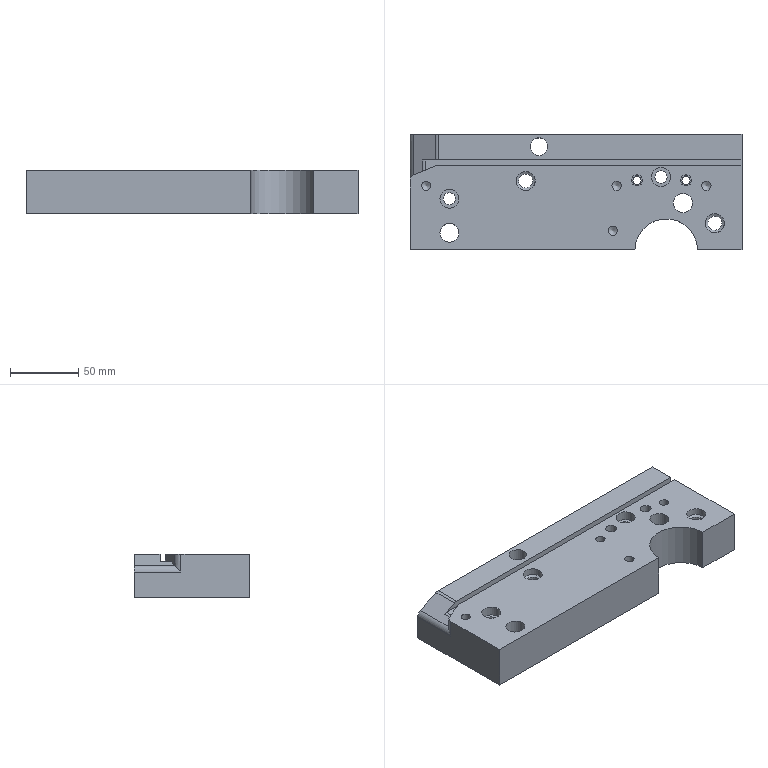Part | STEP file | gslz 2016.10.28-13_id662_x_t | 1 solid | 52 faces | box 244 x 85 x 32 mm | volume 591177 mm3 | cylinder 27 | plane 19 | cone 6 | commonest cylinder face diameters 14 x6 10 x5 6.8 x4 6 x2 8 x2 9 x2